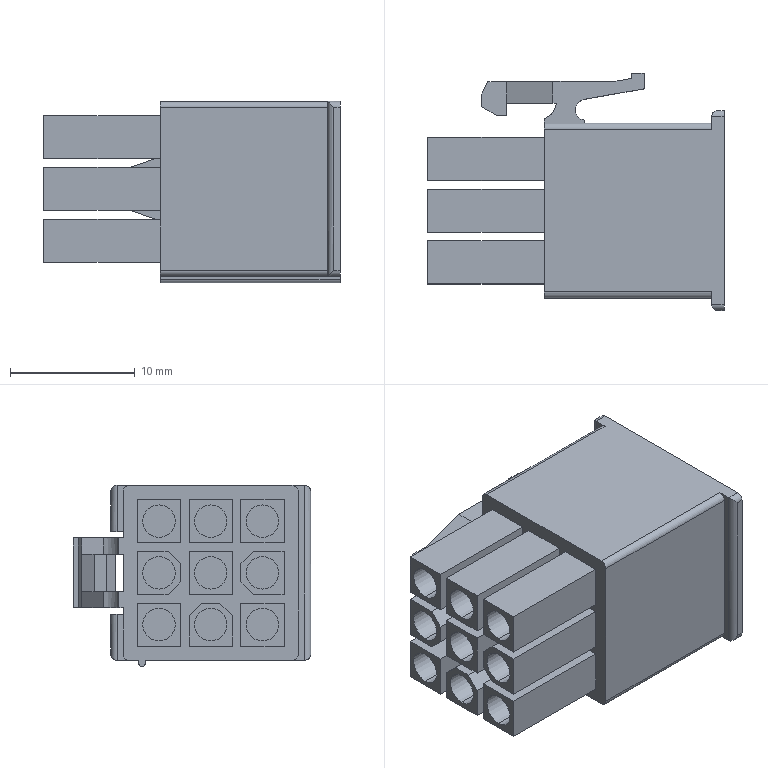Part | STEP file | MHMF_Connector_9_Pin_A6 | 1 solid | 182 faces | box 23.7 x 19 x 14.5 mm | volume 1788 mm3 | plane 148 | cylinder 34 | commonest cylinder face diameters 2.6 x18 1 x11 1.5 x3 0.5 x1 3.1 x1